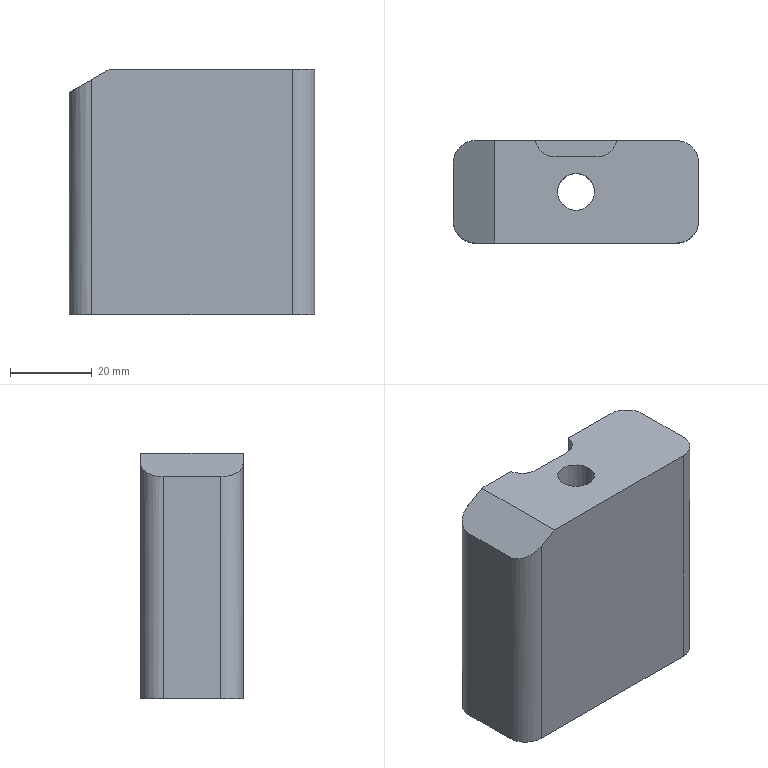Part | NX | features 1605338300 2 | 1 solid | 20 faces | box 60 x 25 x 60 mm | volume 69257 mm3 | plane 11 | cylinder 9 | commonest cylinder face diameters 11 x4 10 x2 17 x2 9 x1
STEP:
#1=CARTESIAN_POINT('',(-66.5,86.,-61.5));
#2=VERTEX_POINT('',#1);
#3=CARTESIAN_POINT('',(-58.,86.,-61.5));
#4=DIRECTION('',(0.,0.,-1.));
#5=DIRECTION('',(-1.,0.,0.));
#6=AXIS2_PLACEMENT_3D('',#3,#4,#5);
#7=CIRCLE('',#6,8.5);
#8=EDGE_CURVE('',#2,#2,#7,.F.);
#9=ORIENTED_EDGE('',*,*,#8,.T.);
#10=EDGE_LOOP('',(#9));
#11=FACE_BOUND('',#10,.T.);
#12=CARTESIAN_POINT('',(-78.5,86.,-61.5));
#13=VERTEX_POINT('',#12);
#14=CARTESIAN_POINT('',(-74.,86.,-61.5));
#15=DIRECTION('',(0.,0.,-1.));
#16=DIRECTION('',(-1.,0.,0.));
#17=AXIS2_PLACEMENT_3D('',#14,#15,#16);
#18=CIRCLE('',#17,4.5);
#19=EDGE_CURVE('',#13,#13,#18,.T.);
#20=ORIENTED_EDGE('',*,*,#19,.F.);
#21=EDGE_LOOP('',(#20));
#22=FACE_BOUND('',#21,.T.);
#23=CARTESIAN_POINT('',(-104.,79.,-61.5));
#24=VERTEX_POINT('',#23);
#25=CARTESIAN_POINT('',(-104.,93.,-61.5));
#26=VERTEX_POINT('',#25);
#27=CARTESIAN_POINT('',(-104.,81.,-61.5));
#28=DIRECTION('',(0.,1.,0.));
#29=VECTOR('',#28,1000.);
#30=LINE('',#27,#29);
#31=EDGE_CURVE('',#24,#26,#30,.T.);
#32=ORIENTED_EDGE('',*,*,#31,.T.);
#33=CARTESIAN_POINT('',(-98.5,98.5,-61.5));
#34=VERTEX_POINT('',#33);
#35=CARTESIAN_POINT('',(-98.5,93.,-61.5));
#36=DIRECTION('',(0.,0.,-1.));
#37=DIRECTION('',(-1.,0.,0.));
#38=AXIS2_PLACEMENT_3D('',#35,#36,#37);
#39=CIRCLE('',#38,5.5);
#40=EDGE_CURVE('',#34,#26,#39,.F.);
#41=ORIENTED_EDGE('',*,*,#40,.F.);
#42=CARTESIAN_POINT('',(-49.5,98.5,-61.5));
#43=VERTEX_POINT('',#42);
#44=CARTESIAN_POINT('',(-89.,98.5,-61.5));
#45=DIRECTION('',(1.,0.,0.));
#46=VECTOR('',#45,1000.);
#47=LINE('',#44,#46);
#48=EDGE_CURVE('',#34,#43,#47,.T.);
#49=ORIENTED_EDGE('',*,*,#48,.T.);
#50=CARTESIAN_POINT('',(-44.,93.,-61.5));
#51=VERTEX_POINT('',#50);
#52=CARTESIAN_POINT('',(-49.5,93.,-61.5));
#53=DIRECTION('',(0.,0.,-1.));
#54=DIRECTION('',(-1.,0.,0.));
#55=AXIS2_PLACEMENT_3D('',#52,#53,#54);
#56=CIRCLE('',#55,5.5);
#57=EDGE_CURVE('',#51,#43,#56,.F.);
#58=ORIENTED_EDGE('',*,*,#57,.F.);
#59=CARTESIAN_POINT('',(-44.,79.,-61.5));
#60=VERTEX_POINT('',#59);
#61=CARTESIAN_POINT('',(-44.,81.,-61.5));
#62=DIRECTION('',(0.,-1.,0.));
#63=VECTOR('',#62,1000.);
#64=LINE('',#61,#63);
#65=EDGE_CURVE('',#51,#60,#64,.T.);
#66=ORIENTED_EDGE('',*,*,#65,.T.);
#67=CARTESIAN_POINT('',(-49.5,73.5,-61.5));
#68=VERTEX_POINT('',#67);
#69=CARTESIAN_POINT('',(-49.5,79.,-61.5));
#70=DIRECTION('',(0.,0.,-1.));
#71=DIRECTION('',(-1.,0.,0.));
#72=AXIS2_PLACEMENT_3D('',#69,#70,#71);
#73=CIRCLE('',#72,5.5);
#74=EDGE_CURVE('',#68,#60,#73,.F.);
#75=ORIENTED_EDGE('',*,*,#74,.F.);
#76=CARTESIAN_POINT('',(-98.5,73.5,-61.5));
#77=VERTEX_POINT('',#76);
#78=CARTESIAN_POINT('',(-89.,73.5,-61.5));
#79=DIRECTION('',(-1.,0.,0.));
#80=VECTOR('',#79,1000.);
#81=LINE('',#78,#80);
#82=EDGE_CURVE('',#68,#77,#81,.T.);
#83=ORIENTED_EDGE('',*,*,#82,.T.);
#84=CARTESIAN_POINT('',(-98.5,79.,-61.5));
#85=DIRECTION('',(0.,0.,-1.));
#86=DIRECTION('',(-1.,0.,0.));
#87=AXIS2_PLACEMENT_3D('',#84,#85,#86);
#88=CIRCLE('',#87,5.5);
#89=EDGE_CURVE('',#24,#77,#88,.F.);
#90=ORIENTED_EDGE('',*,*,#89,.F.);
#91=EDGE_LOOP('',(#32,#41,#49,#58,#66,#75,#83,#90));
#92=FACE_BOUND('',#91,.T.);
#93=CARTESIAN_POINT('',(-98.5,86.,-61.5));
#94=VERTEX_POINT('',#93);
#95=CARTESIAN_POINT('',(-90.,86.,-61.5));
#96=DIRECTION('',(0.,0.,-1.));
#97=DIRECTION('',(-1.,0.,0.));
#98=AXIS2_PLACEMENT_3D('',#95,#96,#97);
#99=CIRCLE('',#98,8.5);
#100=EDGE_CURVE('',#94,#94,#99,.F.);
#101=ORIENTED_EDGE('',*,*,#100,.T.);
#102=EDGE_LOOP('',(#101));
#103=FACE_BOUND('',#102,.T.);
#104=CARTESIAN_POINT('',(-89.,81.,-61.5));
#105=DIRECTION('',(0.,0.,-1.));
#106=DIRECTION('',(-1.,0.,0.));
#107=AXIS2_PLACEMENT_3D('',#104,#105,#106);
#108=PLANE('',#107);
#109=ADVANCED_FACE('',(#11,#22,#92,#103),#108,.T.);
#110=CARTESIAN_POINT('',(-69.5,86.,-1.5));
#111=VERTEX_POINT('',#110);
#112=CARTESIAN_POINT('',(-74.,86.,-1.5));
#113=DIRECTION('',(0.,0.,1.));
#114=DIRECTION('',(1.,0.,0.));
#115=AXIS2_PLACEMENT_3D('',#112,#113,#114);
#116=CIRCLE('',#115,4.5);
#117=EDGE_CURVE('',#111,#111,#116,.F.);
#118=ORIENTED_EDGE('',*,*,#117,.F.);
#119=EDGE_LOOP('',(#118));
#120=FACE_BOUND('',#119,.T.);
#121=ORIENTED_EDGE('',*,*,#19,.T.);
#122=EDGE_LOOP('',(#121));
#123=FACE_BOUND('',#122,.T.);
#124=CARTESIAN_POINT('',(-74.,86.,20.5));
#125=DIRECTION('',(0.,0.,-1.));
#126=DIRECTION('',(-1.,0.,0.));
#127=AXIS2_PLACEMENT_3D('',#124,#125,#126);
#128=CYLINDRICAL_SURFACE('',#127,4.5);
#129=ADVANCED_FACE('',(#120,#123),#128,.F.);
#130=CARTESIAN_POINT('',(-79.101,94.5,-1.5));
#131=VERTEX_POINT('',#130);
#132=CARTESIAN_POINT('',(-68.899,94.5,-1.5));
#133=VERTEX_POINT('',#132);
#134=CARTESIAN_POINT('',(-78.,94.5,-1.5));
#135=DIRECTION('',(1.,0.,0.));
#136=VECTOR('',#135,1000.);
#137=LINE('',#134,#136);
#138=EDGE_CURVE('',#131,#133,#137,.T.);
#139=ORIENTED_EDGE('',*,*,#138,.F.);
#140=CARTESIAN_POINT('',(-84.,98.5,-1.5));
#141=VERTEX_POINT('',#140);
#142=CARTESIAN_POINT('',(-79.101,99.5,-1.5));
#143=DIRECTION('',(0.,0.,-1.));
#144=DIRECTION('',(1.,0.,0.));
#145=AXIS2_PLACEMENT_3D('',#142,#143,#144);
#146=CIRCLE('',#145,5.);
#147=EDGE_CURVE('',#141,#131,#146,.F.);
#148=ORIENTED_EDGE('',*,*,#147,.F.);
#149=CARTESIAN_POINT('',(-94.,98.5,-1.5));
#150=VERTEX_POINT('',#149);
#151=CARTESIAN_POINT('',(-89.,98.5,-1.5));
#152=DIRECTION('',(-1.,0.,0.));
#153=VECTOR('',#152,1000.);
#154=LINE('',#151,#153);
#155=EDGE_CURVE('',#141,#150,#154,.T.);
#156=ORIENTED_EDGE('',*,*,#155,.T.);
#157=CARTESIAN_POINT('',(-94.,73.5,-1.5));
#158=VERTEX_POINT('',#157);
#159=CARTESIAN_POINT('',(-94.,81.,-1.5));
#160=DIRECTION('',(0.,1.,0.));
#161=VECTOR('',#160,1000.);
#162=LINE('',#159,#161);
#163=EDGE_CURVE('',#158,#150,#162,.T.);
#164=ORIENTED_EDGE('',*,*,#163,.F.);
#165=CARTESIAN_POINT('',(-49.5,73.5,-1.5));
#166=VERTEX_POINT('',#165);
#167=CARTESIAN_POINT('',(-89.,73.5,-1.5));
#168=DIRECTION('',(1.,0.,0.));
#169=VECTOR('',#168,1000.);
#170=LINE('',#167,#169);
#171=EDGE_CURVE('',#158,#166,#170,.T.);
#172=ORIENTED_EDGE('',*,*,#171,.T.);
#173=CARTESIAN_POINT('',(-44.,79.,-1.5));
#174=VERTEX_POINT('',#173);
#175=CARTESIAN_POINT('',(-49.5,79.,-1.5));
#176=DIRECTION('',(0.,0.,1.));
#177=DIRECTION('',(1.,0.,0.));
#178=AXIS2_PLACEMENT_3D('',#175,#176,#177);
#179=CIRCLE('',#178,5.5);
#180=EDGE_CURVE('',#174,#166,#179,.F.);
#181=ORIENTED_EDGE('',*,*,#180,.F.);
#182=CARTESIAN_POINT('',(-44.,93.,-1.5));
#183=VERTEX_POINT('',#182);
#184=CARTESIAN_POINT('',(-44.,81.,-1.5));
#185=DIRECTION('',(0.,1.,0.));
#186=VECTOR('',#185,1000.);
#187=LINE('',#184,#186);
#188=EDGE_CURVE('',#174,#183,#187,.T.);
#189=ORIENTED_EDGE('',*,*,#188,.T.);
#190=CARTESIAN_POINT('',(-49.5,98.5,-1.5));
#191=VERTEX_POINT('',#190);
#192=CARTESIAN_POINT('',(-49.5,93.,-1.5));
#193=DIRECTION('',(0.,0.,1.));
#194=DIRECTION('',(1.,0.,0.));
#195=AXIS2_PLACEMENT_3D('',#192,#193,#194);
#196=CIRCLE('',#195,5.5);
#197=EDGE_CURVE('',#191,#183,#196,.F.);
#198=ORIENTED_EDGE('',*,*,#197,.F.);
#199=CARTESIAN_POINT('',(-64.,98.5,-1.5));
#200=VERTEX_POINT('',#199);
#201=CARTESIAN_POINT('',(-89.,98.5,-1.5));
#202=DIRECTION('',(-1.,0.,0.));
#203=VECTOR('',#202,1000.);
#204=LINE('',#201,#203);
#205=EDGE_CURVE('',#191,#200,#204,.T.);
#206=ORIENTED_EDGE('',*,*,#205,.T.);
#207=CARTESIAN_POINT('',(-68.899,99.5,-1.5));
#208=DIRECTION('',(0.,0.,-1.));
#209=DIRECTION('',(1.,0.,0.));
#210=AXIS2_PLACEMENT_3D('',#207,#208,#209);
#211=CIRCLE('',#210,5.);
#212=EDGE_CURVE('',#133,#200,#211,.F.);
#213=ORIENTED_EDGE('',*,*,#212,.F.);
#214=EDGE_LOOP('',(#139,#148,#156,#164,#172,#181,#189,#198,#206,#213));
#215=FACE_BOUND('',#214,.T.);
#216=ORIENTED_EDGE('',*,*,#117,.T.);
#217=EDGE_LOOP('',(#216));
#218=FACE_BOUND('',#217,.T.);
#219=CARTESIAN_POINT('',(-89.,81.,-1.5));
#220=DIRECTION('',(0.,0.,1.));
#221=DIRECTION('',(1.,0.,0.));
#222=AXIS2_PLACEMENT_3D('',#219,#220,#221);
#223=PLANE('',#222);
#224=ADVANCED_FACE('',(#215,#218),#223,.T.);
#225=ORIENTED_EDGE('',*,*,#82,.F.);
#226=CARTESIAN_POINT('',(-49.5,73.5,-1.5));
#227=DIRECTION('',(0.,0.,-1.));
#228=VECTOR('',#227,1000.);
#229=LINE('',#226,#228);
#230=EDGE_CURVE('',#166,#68,#229,.T.);
#231=ORIENTED_EDGE('',*,*,#230,.F.);
#232=ORIENTED_EDGE('',*,*,#171,.F.);
#233=CARTESIAN_POINT('',(-98.5,73.5,-4.098));
#234=VERTEX_POINT('',#233);
#235=CARTESIAN_POINT('',(-94.,73.5,-1.5));
#236=DIRECTION('',(-0.866,0.,-0.5));
#237=VECTOR('',#236,1000.);
#238=LINE('',#235,#237);
#239=EDGE_CURVE('',#234,#158,#238,.F.);
#240=ORIENTED_EDGE('',*,*,#239,.F.);
#241=CARTESIAN_POINT('',(-98.5,73.5,-1.5));
#242=DIRECTION('',(0.,0.,-1.));
#243=VECTOR('',#242,1000.);
#244=LINE('',#241,#243);
#245=EDGE_CURVE('',#77,#234,#244,.F.);
#246=ORIENTED_EDGE('',*,*,#245,.F.);
#247=EDGE_LOOP('',(#225,#231,#232,#240,#246));
#248=FACE_BOUND('',#247,.T.);
#249=CARTESIAN_POINT('',(-89.,73.5,-1.5));
#250=DIRECTION('',(0.,-1.,0.));
#251=DIRECTION('',(0.,0.,1.));
#252=AXIS2_PLACEMENT_3D('',#249,#250,#251);
#253=PLANE('',#252);
#254=ADVANCED_FACE('',(#248),#253,.T.);
#255=CARTESIAN_POINT('',(-104.,93.,-7.274));
#256=VERTEX_POINT('',#255);
#257=CARTESIAN_POINT('',(-104.,79.,-7.274));
#258=VERTEX_POINT('',#257);
#259=CARTESIAN_POINT('',(-104.,81.,-7.274));
#260=DIRECTION('',(0.,-1.,0.));
#261=VECTOR('',#260,1000.);
#262=LINE('',#259,#261);
#263=EDGE_CURVE('',#256,#258,#262,.T.);
#264=ORIENTED_EDGE('',*,*,#263,.F.);
#265=CARTESIAN_POINT('',(-104.,93.,-1.5));
#266=DIRECTION('',(0.,0.,-1.));
#267=VECTOR('',#266,1000.);
#268=LINE('',#265,#267);
#269=EDGE_CURVE('',#26,#256,#268,.F.);
#270=ORIENTED_EDGE('',*,*,#269,.F.);
#271=ORIENTED_EDGE('',*,*,#31,.F.);
#272=CARTESIAN_POINT('',(-104.,79.,-1.5));
#273=DIRECTION('',(0.,0.,-1.));
#274=VECTOR('',#273,1000.);
#275=LINE('',#272,#274);
#276=EDGE_CURVE('',#258,#24,#275,.T.);
#277=ORIENTED_EDGE('',*,*,#276,.F.);
#278=EDGE_LOOP('',(#264,#270,#271,#277));
#279=FACE_BOUND('',#278,.T.);
#280=CARTESIAN_POINT('',(-104.,81.,-1.5));
#281=DIRECTION('',(-1.,0.,0.));
#282=DIRECTION('',(0.,0.,1.));
#283=AXIS2_PLACEMENT_3D('',#280,#281,#282);
#284=PLANE('',#283);
#285=ADVANCED_FACE('',(#279),#284,.T.);
#286=CARTESIAN_POINT('',(-84.,98.5,-36.5));
#287=VERTEX_POINT('',#286);
#288=CARTESIAN_POINT('',(-84.,98.5,-1.5));
#289=DIRECTION('',(0.,0.,-1.));
#290=VECTOR('',#289,1000.);
#291=LINE('',#288,#290);
#292=EDGE_CURVE('',#141,#287,#291,.T.);
#293=ORIENTED_EDGE('',*,*,#292,.T.);
#294=CARTESIAN_POINT('',(-64.,98.5,-36.5));
#295=VERTEX_POINT('',#294);
#296=CARTESIAN_POINT('',(-89.,98.5,-36.5));
#297=DIRECTION('',(1.,0.,0.));
#298=VECTOR('',#297,1000.);
#299=LINE('',#296,#298);
#300=EDGE_CURVE('',#287,#295,#299,.T.);
#301=ORIENTED_EDGE('',*,*,#300,.T.);
#302=CARTESIAN_POINT('',(-64.,98.5,-1.5));
#303=DIRECTION('',(0.,0.,1.));
#304=VECTOR('',#303,1000.);
#305=LINE('',#302,#304);
#306=EDGE_CURVE('',#295,#200,#305,.T.);
#307=ORIENTED_EDGE('',*,*,#306,.T.);
#308=ORIENTED_EDGE('',*,*,#205,.F.);
#309=CARTESIAN_POINT('',(-49.5,98.5,-1.5));
#310=DIRECTION('',(0.,0.,-1.));
#311=VECTOR('',#310,1000.);
#312=LINE('',#309,#311);
#313=EDGE_CURVE('',#43,#191,#312,.F.);
#314=ORIENTED_EDGE('',*,*,#313,.F.);
#315=ORIENTED_EDGE('',*,*,#48,.F.);
#316=CARTESIAN_POINT('',(-98.5,98.5,-4.098));
#317=VERTEX_POINT('',#316);
#318=CARTESIAN_POINT('',(-98.5,98.5,-1.5));
#319=DIRECTION('',(0.,0.,-1.));
#320=VECTOR('',#319,1000.);
#321=LINE('',#318,#320);
#322=EDGE_CURVE('',#317,#34,#321,.T.);
#323=ORIENTED_EDGE('',*,*,#322,.F.);
#324=CARTESIAN_POINT('',(-94.,98.5,-1.5));
#325=DIRECTION('',(0.866,0.,0.5));
#326=VECTOR('',#325,1000.);
#327=LINE('',#324,#326);
#328=EDGE_CURVE('',#150,#317,#327,.F.);
#329=ORIENTED_EDGE('',*,*,#328,.F.);
#330=ORIENTED_EDGE('',*,*,#155,.F.);
#331=EDGE_LOOP('',(#293,#301,#307,#308,#314,#315,#323,#329,#330));
#332=FACE_BOUND('',#331,.T.);
#333=CARTESIAN_POINT('',(-89.,98.5,-1.5));
#334=DIRECTION('',(0.,1.,0.));
#335=DIRECTION('',(0.,0.,-1.));
#336=AXIS2_PLACEMENT_3D('',#333,#334,#335);
#337=PLANE('',#336);
#338=ADVANCED_FACE('',(#332),#337,.T.);
#339=ORIENTED_EDGE('',*,*,#65,.F.);
#340=CARTESIAN_POINT('',(-44.,93.,-1.5));
#341=DIRECTION('',(0.,0.,-1.));
#342=VECTOR('',#341,1000.);
#343=LINE('',#340,#342);
#344=EDGE_CURVE('',#183,#51,#343,.T.);
#345=ORIENTED_EDGE('',*,*,#344,.F.);
#346=ORIENTED_EDGE('',*,*,#188,.F.);
#347=CARTESIAN_POINT('',(-44.,79.,-1.5));
#348=DIRECTION('',(0.,0.,-1.));
#349=VECTOR('',#348,1000.);
#350=LINE('',#347,#349);
#351=EDGE_CURVE('',#60,#174,#350,.F.);
#352=ORIENTED_EDGE('',*,*,#351,.F.);
#353=EDGE_LOOP('',(#339,#345,#346,#352));
#354=FACE_BOUND('',#353,.T.);
#355=CARTESIAN_POINT('',(-44.,81.,-1.5));
#356=DIRECTION('',(1.,0.,0.));
#357=DIRECTION('',(0.,0.,-1.));
#358=AXIS2_PLACEMENT_3D('',#355,#356,#357);
#359=PLANE('',#358);
#360=ADVANCED_FACE('',(#354),#359,.T.);
#361=ORIENTED_EDGE('',*,*,#239,.T.);
#362=ORIENTED_EDGE('',*,*,#163,.T.);
#363=ORIENTED_EDGE('',*,*,#328,.T.);
#364=CARTESIAN_POINT('',(-98.5,93.,-4.098));
#365=DIRECTION('',(0.5,0.,-0.866));
#366=DIRECTION('',(0.866,0.,0.5));
#367=AXIS2_PLACEMENT_3D('',#364,#365,#366);
#368=ELLIPSE('',#367,6.351,5.5);
#369=EDGE_CURVE('',#256,#317,#368,.T.);
#370=ORIENTED_EDGE('',*,*,#369,.F.);
#371=ORIENTED_EDGE('',*,*,#263,.T.);
#372=CARTESIAN_POINT('',(-98.5,79.,-4.098));
#373=DIRECTION('',(0.5,0.,-0.866));
#374=DIRECTION('',(0.866,0.,0.5));
#375=AXIS2_PLACEMENT_3D('',#372,#373,#374);
#376=ELLIPSE('',#375,6.351,5.5);
#377=EDGE_CURVE('',#234,#258,#376,.T.);
#378=ORIENTED_EDGE('',*,*,#377,.F.);
#379=EDGE_LOOP('',(#361,#362,#363,#370,#371,#378));
#380=FACE_BOUND('',#379,.T.);
#381=CARTESIAN_POINT('',(-104.,81.,-7.274));
#382=DIRECTION('',(0.5,0.,-0.866));
#383=DIRECTION('',(-0.866,0.,-0.5));
#384=AXIS2_PLACEMENT_3D('',#381,#382,#383);
#385=PLANE('',#384);
#386=ADVANCED_FACE('',(#380),#385,.F.);
#387=ORIENTED_EDGE('',*,*,#197,.T.);
#388=ORIENTED_EDGE('',*,*,#344,.T.);
#389=ORIENTED_EDGE('',*,*,#57,.T.);
#390=ORIENTED_EDGE('',*,*,#313,.T.);
#391=EDGE_LOOP('',(#387,#388,#389,#390));
#392=FACE_BOUND('',#391,.T.);
#393=CARTESIAN_POINT('',(-49.5,93.,-1.5));
#394=DIRECTION('',(0.,0.,1.));
#395=DIRECTION('',(1.,0.,0.));
#396=AXIS2_PLACEMENT_3D('',#393,#394,#395);
#397=CYLINDRICAL_SURFACE('',#396,5.5);
#398=ADVANCED_FACE('',(#392),#397,.T.);
#399=ORIENTED_EDGE('',*,*,#180,.T.);
#400=ORIENTED_EDGE('',*,*,#230,.T.);
#401=ORIENTED_EDGE('',*,*,#74,.T.);
#402=ORIENTED_EDGE('',*,*,#351,.T.);
#403=EDGE_LOOP('',(#399,#400,#401,#402));
#404=FACE_BOUND('',#403,.T.);
#405=CARTESIAN_POINT('',(-49.5,79.,-1.5));
#406=DIRECTION('',(0.,0.,1.));
#407=DIRECTION('',(1.,0.,0.));
#408=AXIS2_PLACEMENT_3D('',#405,#406,#407);
#409=CYLINDRICAL_SURFACE('',#408,5.5);
#410=ADVANCED_FACE('',(#404),#409,.T.);
#411=ORIENTED_EDGE('',*,*,#369,.T.);
#412=ORIENTED_EDGE('',*,*,#322,.T.);
#413=ORIENTED_EDGE('',*,*,#40,.T.);
#414=ORIENTED_EDGE('',*,*,#269,.T.);
#415=EDGE_LOOP('',(#411,#412,#413,#414));
#416=FACE_BOUND('',#415,.T.);
#417=CARTESIAN_POINT('',(-98.5,93.,-1.5));
#418=DIRECTION('',(0.,0.,1.));
#419=DIRECTION('',(1.,0.,0.));
#420=AXIS2_PLACEMENT_3D('',#417,#418,#419);
#421=CYLINDRICAL_SURFACE('',#420,5.5);
#422=ADVANCED_FACE('',(#416),#421,.T.);
#423=ORIENTED_EDGE('',*,*,#377,.T.);
#424=ORIENTED_EDGE('',*,*,#276,.T.);
#425=ORIENTED_EDGE('',*,*,#89,.T.);
#426=ORIENTED_EDGE('',*,*,#245,.T.);
#427=EDGE_LOOP('',(#423,#424,#425,#426));
#428=FACE_BOUND('',#427,.T.);
#429=CARTESIAN_POINT('',(-98.5,79.,-1.5));
#430=DIRECTION('',(0.,0.,1.));
#431=DIRECTION('',(1.,0.,0.));
#432=AXIS2_PLACEMENT_3D('',#429,#430,#431);
#433=CYLINDRICAL_SURFACE('',#432,5.5);
#434=ADVANCED_FACE('',(#428),#433,.T.);
#435=CARTESIAN_POINT('',(-79.101,94.5,-36.5));
#436=VERTEX_POINT('',#435);
#437=CARTESIAN_POINT('',(-68.899,94.5,-36.5));
#438=VERTEX_POINT('',#437);
#439=CARTESIAN_POINT('',(-82.,94.5,-36.5));
#440=DIRECTION('',(1.,0.,0.));
#441=VECTOR('',#440,1000.);
#442=LINE('',#439,#441);
#443=EDGE_CURVE('',#436,#438,#442,.T.);
#444=ORIENTED_EDGE('',*,*,#443,.F.);
#445=CARTESIAN_POINT('',(-79.101,94.5,-16.5));
#446=DIRECTION('',(0.,0.,1.));
#447=VECTOR('',#446,1000.);
#448=LINE('',#445,#447);
#449=EDGE_CURVE('',#131,#436,#448,.F.);
#450=ORIENTED_EDGE('',*,*,#449,.F.);
#451=ORIENTED_EDGE('',*,*,#138,.T.);
#452=CARTESIAN_POINT('',(-68.899,94.5,-16.5));
#453=DIRECTION('',(0.,0.,-1.));
#454=VECTOR('',#453,1000.);
#455=LINE('',#452,#454);
#456=EDGE_CURVE('',#438,#133,#455,.F.);
#457=ORIENTED_EDGE('',*,*,#456,.F.);
#458=EDGE_LOOP('',(#444,#450,#451,#457));
#459=FACE_BOUND('',#458,.T.);
#460=CARTESIAN_POINT('',(-78.,94.5,-16.5));
#461=DIRECTION('',(0.,-1.,0.));
#462=DIRECTION('',(0.,0.,1.));
#463=AXIS2_PLACEMENT_3D('',#460,#461,#462);
#464=PLANE('',#463);
#465=ADVANCED_FACE('',(#459),#464,.F.);
#466=ORIENTED_EDGE('',*,*,#300,.F.);
#467=CARTESIAN_POINT('',(-79.101,99.5,-36.5));
#468=DIRECTION('',(0.,0.,1.));
#469=DIRECTION('',(1.,0.,0.));
#470=AXIS2_PLACEMENT_3D('',#467,#468,#469);
#471=CIRCLE('',#470,5.);
#472=EDGE_CURVE('',#436,#287,#471,.F.);
#473=ORIENTED_EDGE('',*,*,#472,.F.);
#474=ORIENTED_EDGE('',*,*,#443,.T.);
#475=CARTESIAN_POINT('',(-68.899,99.5,-36.5));
#476=DIRECTION('',(0.,0.,1.));
#477=DIRECTION('',(1.,0.,0.));
#478=AXIS2_PLACEMENT_3D('',#475,#476,#477);
#479=CIRCLE('',#478,5.);
#480=EDGE_CURVE('',#295,#438,#479,.F.);
#481=ORIENTED_EDGE('',*,*,#480,.F.);
#482=EDGE_LOOP('',(#466,#473,#474,#481));
#483=FACE_BOUND('',#482,.T.);
#484=CARTESIAN_POINT('',(-82.,98.5,-36.5));
#485=DIRECTION('',(0.,0.,1.));
#486=DIRECTION('',(1.,0.,0.));
#487=AXIS2_PLACEMENT_3D('',#484,#485,#486);
#488=PLANE('',#487);
#489=ADVANCED_FACE('',(#483),#488,.T.);
#490=ORIENTED_EDGE('',*,*,#472,.T.);
#491=ORIENTED_EDGE('',*,*,#292,.F.);
#492=ORIENTED_EDGE('',*,*,#147,.T.);
#493=ORIENTED_EDGE('',*,*,#449,.T.);
#494=EDGE_LOOP('',(#490,#491,#492,#493));
#495=FACE_BOUND('',#494,.T.);
#496=CARTESIAN_POINT('',(-79.101,99.5,-16.5));
#497=DIRECTION('',(0.,0.,1.));
#498=DIRECTION('',(1.,0.,0.));
#499=AXIS2_PLACEMENT_3D('',#496,#497,#498);
#500=CYLINDRICAL_SURFACE('',#499,5.);
#501=ADVANCED_FACE('',(#495),#500,.F.);
#502=ORIENTED_EDGE('',*,*,#480,.T.);
#503=ORIENTED_EDGE('',*,*,#456,.T.);
#504=ORIENTED_EDGE('',*,*,#212,.T.);
#505=ORIENTED_EDGE('',*,*,#306,.F.);
#506=EDGE_LOOP('',(#502,#503,#504,#505));
#507=FACE_BOUND('',#506,.T.);
#508=CARTESIAN_POINT('',(-68.899,99.5,-16.5));
#509=DIRECTION('',(0.,0.,-1.));
#510=DIRECTION('',(-1.,0.,0.));
#511=AXIS2_PLACEMENT_3D('',#508,#509,#510);
#512=CYLINDRICAL_SURFACE('',#511,5.);
#513=ADVANCED_FACE('',(#507),#512,.F.);
#514=ORIENTED_EDGE('',*,*,#8,.F.);
#515=EDGE_LOOP('',(#514));
#516=FACE_BOUND('',#515,.T.);
#517=CARTESIAN_POINT('',(-66.5,86.,-34.5));
#518=VERTEX_POINT('',#517);
#519=CARTESIAN_POINT('',(-58.,86.,-34.5));
#520=DIRECTION('',(0.,0.,-1.));
#521=DIRECTION('',(-1.,0.,0.));
#522=AXIS2_PLACEMENT_3D('',#519,#520,#521);
#523=CIRCLE('',#522,8.5);
#524=EDGE_CURVE('',#518,#518,#523,.T.);
#525=ORIENTED_EDGE('',*,*,#524,.F.);
#526=EDGE_LOOP('',(#525));
#527=FACE_BOUND('',#526,.T.);
#528=CARTESIAN_POINT('',(-58.,86.,-34.5));
#529=DIRECTION('',(0.,0.,-1.));
#530=DIRECTION('',(-1.,0.,0.));
#531=AXIS2_PLACEMENT_3D('',#528,#529,#530);
#532=CYLINDRICAL_SURFACE('',#531,8.5);
#533=ADVANCED_FACE('',(#516,#527),#532,.F.);
#534=ORIENTED_EDGE('',*,*,#524,.T.);
#535=EDGE_LOOP('',(#534));
#536=FACE_BOUND('',#535,.T.);
#537=CARTESIAN_POINT('',(-108.,21.5,-34.5));
#538=DIRECTION('',(0.,0.,-1.));
#539=DIRECTION('',(-1.,0.,0.));
#540=AXIS2_PLACEMENT_3D('',#537,#538,#539);
#541=PLANE('',#540);
#542=ADVANCED_FACE('',(#536),#541,.T.);
#543=ORIENTED_EDGE('',*,*,#100,.F.);
#544=EDGE_LOOP('',(#543));
#545=FACE_BOUND('',#544,.T.);
#546=CARTESIAN_POINT('',(-98.5,86.,-34.5));
#547=VERTEX_POINT('',#546);
#548=CARTESIAN_POINT('',(-90.,86.,-34.5));
#549=DIRECTION('',(0.,0.,-1.));
#550=DIRECTION('',(-1.,0.,0.));
#551=AXIS2_PLACEMENT_3D('',#548,#549,#550);
#552=CIRCLE('',#551,8.5);
#553=EDGE_CURVE('',#547,#547,#552,.T.);
#554=ORIENTED_EDGE('',*,*,#553,.F.);
#555=EDGE_LOOP('',(#554));
#556=FACE_BOUND('',#555,.T.);
#557=CARTESIAN_POINT('',(-90.,86.,-34.5));
#558=DIRECTION('',(0.,0.,-1.));
#559=DIRECTION('',(-1.,0.,0.));
#560=AXIS2_PLACEMENT_3D('',#557,#558,#559);
#561=CYLINDRICAL_SURFACE('',#560,8.5);
#562=ADVANCED_FACE('',(#545,#556),#561,.F.);
#563=ORIENTED_EDGE('',*,*,#553,.T.);
#564=EDGE_LOOP('',(#563));
#565=FACE_BOUND('',#564,.T.);
#566=CARTESIAN_POINT('',(-140.,21.5,-34.5));
#567=DIRECTION('',(0.,0.,-1.));
#568=DIRECTION('',(-1.,0.,0.));
#569=AXIS2_PLACEMENT_3D('',#566,#567,#568);
#570=PLANE('',#569);
#571=ADVANCED_FACE('',(#565),#570,.T.);
#572=CLOSED_SHELL('',(#109,#129,#224,#254,#285,#338,#360,#386,#398,#410,#422,#434,#465,#489,#501,#513,#533,#542,#562,#571));
#573=MANIFOLD_SOLID_BREP('',#572);
#574=(LENGTH_UNIT()NAMED_UNIT(*)SI_UNIT(.MILLI.,.METRE.));
#575=UNCERTAINTY_MEASURE_WITH_UNIT(LENGTH_MEASURE(0.00001),#574,'','');
#576=(NAMED_UNIT(*)PLANE_ANGLE_UNIT()SI_UNIT($,.RADIAN.));
#577=(NAMED_UNIT(*)SI_UNIT($,.STERADIAN.)SOLID_ANGLE_UNIT());
#578=(GEOMETRIC_REPRESENTATION_CONTEXT(3)GLOBAL_UNCERTAINTY_ASSIGNED_CONTEXT((#575))GLOBAL_UNIT_ASSIGNED_CONTEXT((#574,#576,#577))REPRESENTATION_CONTEXT('',''));
#579=ADVANCED_BREP_SHAPE_REPRESENTATION('',(#573),#578);